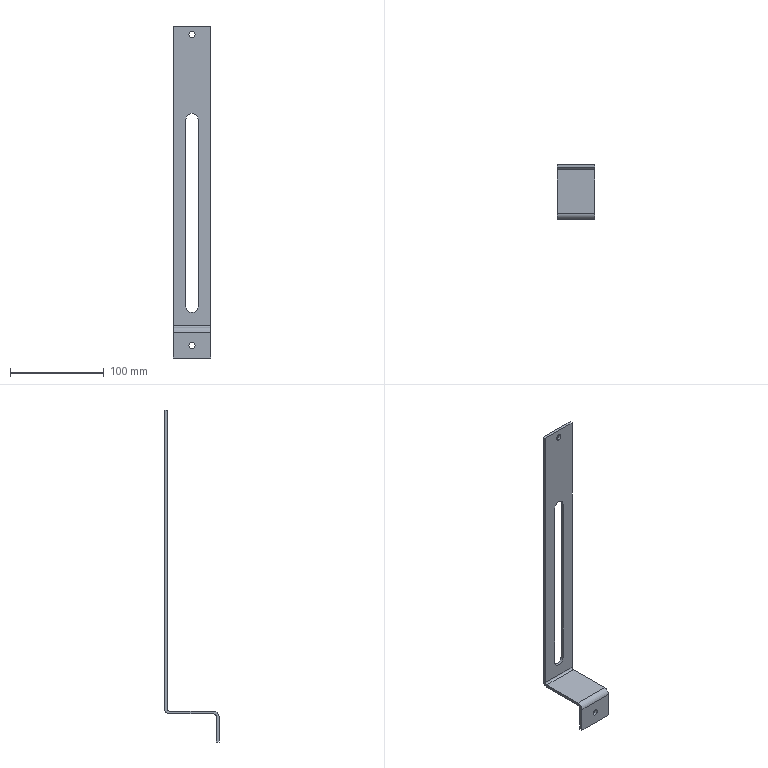Part | STEP file | PN_0028 Sensor switch bracket | 1 solid | 23 faces | box 40 x 58 x 355 mm | volume 40391 mm3 | plane 12 | cylinder 11 | commonest cylinder face diameters 6.5 x4 13 x3 4 x1 6 x1 10 x1 12 x1